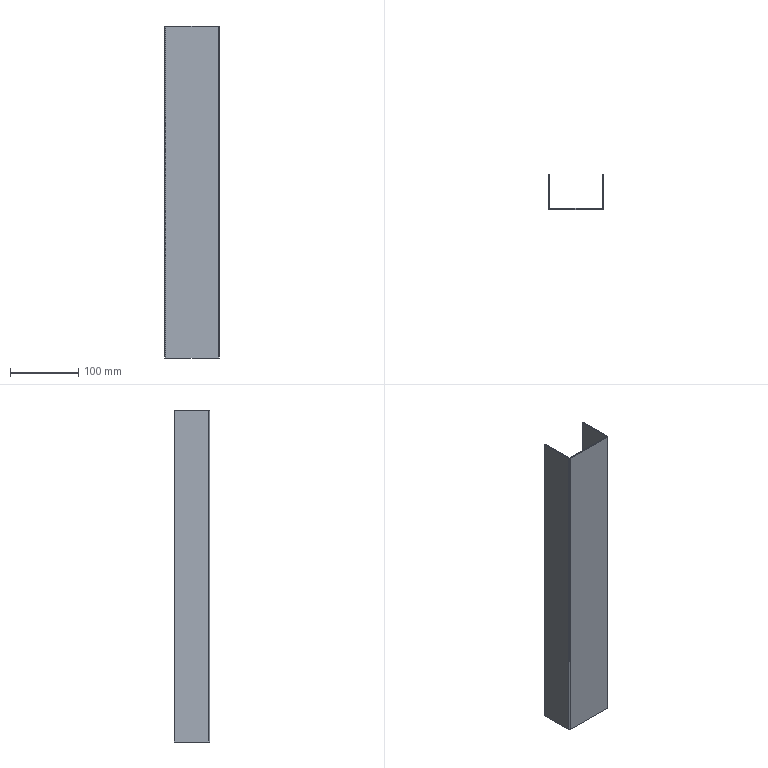Part | SolidWorks | features SplitBody 1 | 1 solid | 22 faces | box 80 x 51.5 x 487 mm | volume 130957 mm3 | plane 18 | cylinder 4 | commonest cylinder face diameters 0.2 x2 3.2 x2
STEP:
#1=CARTESIAN_POINT('',(40.,-51.4,-243.5));
#2=VERTEX_POINT('',#1);
#3=CARTESIAN_POINT('',(38.5,-51.4,-243.5));
#4=VERTEX_POINT('',#3);
#5=CARTESIAN_POINT('',(40.,-51.4,-243.5));
#6=DIRECTION('',(-1.,0.,0.));
#7=VECTOR('',#6,1000.);
#8=LINE('',#5,#7);
#9=EDGE_CURVE('',#2,#4,#8,.T.);
#10=ORIENTED_EDGE('',*,*,#9,.F.);
#11=CARTESIAN_POINT('',(38.4,-53.,-243.5));
#12=VERTEX_POINT('',#11);
#13=CARTESIAN_POINT('',(38.4,-51.4,-243.5));
#14=DIRECTION('',(0.,0.,-1.));
#15=DIRECTION('',(1.,0.,0.));
#16=AXIS2_PLACEMENT_3D('',#13,#14,#15);
#17=CIRCLE('',#16,1.6);
#18=EDGE_CURVE('',#2,#12,#17,.T.);
#19=ORIENTED_EDGE('',*,*,#18,.T.);
#20=CARTESIAN_POINT('',(38.4,-51.5,-243.5));
#21=VERTEX_POINT('',#20);
#22=CARTESIAN_POINT('',(38.4,-51.5,-243.5));
#23=DIRECTION('',(0.,-1.,0.));
#24=VECTOR('',#23,1000.);
#25=LINE('',#22,#24);
#26=EDGE_CURVE('',#21,#12,#25,.T.);
#27=ORIENTED_EDGE('',*,*,#26,.F.);
#28=CARTESIAN_POINT('',(38.4,-51.4,-243.5));
#29=DIRECTION('',(0.,0.,-1.));
#30=DIRECTION('',(1.,0.,0.));
#31=AXIS2_PLACEMENT_3D('',#28,#29,#30);
#32=CIRCLE('',#31,0.1);
#33=EDGE_CURVE('',#4,#21,#32,.T.);
#34=ORIENTED_EDGE('',*,*,#33,.F.);
#35=EDGE_LOOP('',(#10,#19,#27,#34));
#36=FACE_OUTER_BOUND('',#35,.T.);
#37=CARTESIAN_POINT('',(40.,-51.4,-243.5));
#38=DIRECTION('',(0.,0.,-1.));
#39=DIRECTION('',(-1.,0.,0.));
#40=AXIS2_PLACEMENT_3D('',#37,#38,#39);
#41=PLANE('',#40);
#42=ADVANCED_FACE('',(#36),#41,.T.);
#43=CARTESIAN_POINT('',(40.,-1.5,-243.5));
#44=VERTEX_POINT('',#43);
#45=CARTESIAN_POINT('',(40.,-53.,-243.5));
#46=DIRECTION('',(0.,-1.,0.));
#47=VECTOR('',#46,1000.);
#48=LINE('',#45,#47);
#49=EDGE_CURVE('',#44,#2,#48,.T.);
#50=ORIENTED_EDGE('',*,*,#49,.T.);
#51=ORIENTED_EDGE('',*,*,#9,.T.);
#52=CARTESIAN_POINT('',(38.5,-1.5,-243.5));
#53=VERTEX_POINT('',#52);
#54=CARTESIAN_POINT('',(38.5,-53.,-243.5));
#55=DIRECTION('',(0.,-1.,0.));
#56=VECTOR('',#55,1000.);
#57=LINE('',#54,#56);
#58=EDGE_CURVE('',#53,#4,#57,.T.);
#59=ORIENTED_EDGE('',*,*,#58,.F.);
#60=CARTESIAN_POINT('',(38.5,-1.5,-243.5));
#61=DIRECTION('',(1.,0.,0.));
#62=VECTOR('',#61,1000.);
#63=LINE('',#60,#62);
#64=EDGE_CURVE('',#53,#44,#63,.T.);
#65=ORIENTED_EDGE('',*,*,#64,.T.);
#66=EDGE_LOOP('',(#50,#51,#59,#65));
#67=FACE_OUTER_BOUND('',#66,.T.);
#68=CARTESIAN_POINT('',(38.4,-51.5,-243.5));
#69=DIRECTION('',(0.,0.,-1.));
#70=DIRECTION('',(-1.,0.,0.));
#71=AXIS2_PLACEMENT_3D('',#68,#69,#70);
#72=PLANE('',#71);
#73=ADVANCED_FACE('',(#67),#72,.T.);
#74=CARTESIAN_POINT('',(-38.4,-53.,-243.5));
#75=VERTEX_POINT('',#74);
#76=CARTESIAN_POINT('',(-38.4,-51.5,-243.5));
#77=VERTEX_POINT('',#76);
#78=CARTESIAN_POINT('',(-38.4,-53.,-243.5));
#79=DIRECTION('',(0.,1.,0.));
#80=VECTOR('',#79,1000.);
#81=LINE('',#78,#80);
#82=EDGE_CURVE('',#75,#77,#81,.T.);
#83=ORIENTED_EDGE('',*,*,#82,.F.);
#84=CARTESIAN_POINT('',(-40.,-51.4,-243.5));
#85=VERTEX_POINT('',#84);
#86=CARTESIAN_POINT('',(-38.4,-51.4,-243.5));
#87=DIRECTION('',(0.,0.,-1.));
#88=DIRECTION('',(1.,0.,0.));
#89=AXIS2_PLACEMENT_3D('',#86,#87,#88);
#90=CIRCLE('',#89,1.6);
#91=EDGE_CURVE('',#75,#85,#90,.T.);
#92=ORIENTED_EDGE('',*,*,#91,.T.);
#93=CARTESIAN_POINT('',(-38.5,-51.4,-243.5));
#94=VERTEX_POINT('',#93);
#95=CARTESIAN_POINT('',(-38.5,-51.4,-243.5));
#96=DIRECTION('',(-1.,0.,0.));
#97=VECTOR('',#96,1000.);
#98=LINE('',#95,#97);
#99=EDGE_CURVE('',#94,#85,#98,.T.);
#100=ORIENTED_EDGE('',*,*,#99,.F.);
#101=CARTESIAN_POINT('',(-38.4,-51.4,-243.5));
#102=DIRECTION('',(0.,0.,-1.));
#103=DIRECTION('',(1.,0.,0.));
#104=AXIS2_PLACEMENT_3D('',#101,#102,#103);
#105=CIRCLE('',#104,0.1);
#106=EDGE_CURVE('',#77,#94,#105,.T.);
#107=ORIENTED_EDGE('',*,*,#106,.F.);
#108=EDGE_LOOP('',(#83,#92,#100,#107));
#109=FACE_OUTER_BOUND('',#108,.T.);
#110=CARTESIAN_POINT('',(-38.4,-53.,-243.5));
#111=DIRECTION('',(0.,0.,-1.));
#112=DIRECTION('',(-1.,0.,0.));
#113=AXIS2_PLACEMENT_3D('',#110,#111,#112);
#114=PLANE('',#113);
#115=ADVANCED_FACE('',(#109),#114,.T.);
#116=CARTESIAN_POINT('',(-40.,-53.,-243.5));
#117=DIRECTION('',(-1.,0.,0.));
#118=VECTOR('',#117,1000.);
#119=LINE('',#116,#118);
#120=EDGE_CURVE('',#12,#75,#119,.T.);
#121=ORIENTED_EDGE('',*,*,#120,.T.);
#122=ORIENTED_EDGE('',*,*,#82,.T.);
#123=CARTESIAN_POINT('',(-40.,-51.5,-243.5));
#124=DIRECTION('',(-1.,0.,0.));
#125=VECTOR('',#124,1000.);
#126=LINE('',#123,#125);
#127=EDGE_CURVE('',#21,#77,#126,.T.);
#128=ORIENTED_EDGE('',*,*,#127,.F.);
#129=ORIENTED_EDGE('',*,*,#26,.T.);
#130=EDGE_LOOP('',(#121,#122,#128,#129));
#131=FACE_OUTER_BOUND('',#130,.T.);
#132=CARTESIAN_POINT('',(-38.5,-51.4,-243.5));
#133=DIRECTION('',(0.,0.,-1.));
#134=DIRECTION('',(-1.,0.,0.));
#135=AXIS2_PLACEMENT_3D('',#132,#133,#134);
#136=PLANE('',#135);
#137=ADVANCED_FACE('',(#131),#136,.T.);
#138=CARTESIAN_POINT('',(-38.5,-51.4,243.5));
#139=VERTEX_POINT('',#138);
#140=CARTESIAN_POINT('',(-38.5,-1.5,243.5));
#141=VERTEX_POINT('',#140);
#142=CARTESIAN_POINT('',(-38.5,-53.,243.5));
#143=DIRECTION('',(0.,1.,0.));
#144=VECTOR('',#143,1000.);
#145=LINE('',#142,#144);
#146=EDGE_CURVE('',#139,#141,#145,.T.);
#147=ORIENTED_EDGE('',*,*,#146,.F.);
#148=CARTESIAN_POINT('',(-38.5,-51.4,338.643));
#149=DIRECTION('',(0.,0.,-1.));
#150=VECTOR('',#149,1000.);
#151=LINE('',#148,#150);
#152=EDGE_CURVE('',#139,#94,#151,.T.);
#153=ORIENTED_EDGE('',*,*,#152,.T.);
#154=CARTESIAN_POINT('',(-38.5,-1.5,-243.5));
#155=VERTEX_POINT('',#154);
#156=CARTESIAN_POINT('',(-38.5,-53.,-243.5));
#157=DIRECTION('',(0.,1.,0.));
#158=VECTOR('',#157,1000.);
#159=LINE('',#156,#158);
#160=EDGE_CURVE('',#94,#155,#159,.T.);
#161=ORIENTED_EDGE('',*,*,#160,.T.);
#162=CARTESIAN_POINT('',(-38.5,-1.5,338.643));
#163=DIRECTION('',(0.,0.,-1.));
#164=VECTOR('',#163,1000.);
#165=LINE('',#162,#164);
#166=EDGE_CURVE('',#141,#155,#165,.T.);
#167=ORIENTED_EDGE('',*,*,#166,.F.);
#168=EDGE_LOOP('',(#147,#153,#161,#167));
#169=FACE_OUTER_BOUND('',#168,.T.);
#170=CARTESIAN_POINT('',(-38.5,-53.,338.643));
#171=DIRECTION('',(-1.,0.,0.));
#172=DIRECTION('',(0.,-1.,0.));
#173=AXIS2_PLACEMENT_3D('',#170,#171,#172);
#174=PLANE('',#173);
#175=ADVANCED_FACE('',(#169),#174,.F.);
#176=CARTESIAN_POINT('',(-40.,-1.5,243.5));
#177=VERTEX_POINT('',#176);
#178=CARTESIAN_POINT('',(-40.,-1.5,-243.5));
#179=VERTEX_POINT('',#178);
#180=CARTESIAN_POINT('',(-40.,-1.5,338.643));
#181=DIRECTION('',(0.,0.,-1.));
#182=VECTOR('',#181,1000.);
#183=LINE('',#180,#182);
#184=EDGE_CURVE('',#177,#179,#183,.T.);
#185=ORIENTED_EDGE('',*,*,#184,.F.);
#186=CARTESIAN_POINT('',(-40.,-1.5,243.5));
#187=DIRECTION('',(1.,0.,0.));
#188=VECTOR('',#187,1000.);
#189=LINE('',#186,#188);
#190=EDGE_CURVE('',#177,#141,#189,.T.);
#191=ORIENTED_EDGE('',*,*,#190,.T.);
#192=ORIENTED_EDGE('',*,*,#166,.T.);
#193=CARTESIAN_POINT('',(-40.,-1.5,-243.5));
#194=DIRECTION('',(1.,0.,0.));
#195=VECTOR('',#194,1000.);
#196=LINE('',#193,#195);
#197=EDGE_CURVE('',#179,#155,#196,.T.);
#198=ORIENTED_EDGE('',*,*,#197,.F.);
#199=EDGE_LOOP('',(#185,#191,#192,#198));
#200=FACE_OUTER_BOUND('',#199,.T.);
#201=CARTESIAN_POINT('',(-40.,-1.5,338.643));
#202=DIRECTION('',(0.,1.,0.));
#203=DIRECTION('',(-1.,0.,0.));
#204=AXIS2_PLACEMENT_3D('',#201,#202,#203);
#205=PLANE('',#204);
#206=ADVANCED_FACE('',(#200),#205,.T.);
#207=CARTESIAN_POINT('',(-40.,-51.4,243.5));
#208=VERTEX_POINT('',#207);
#209=CARTESIAN_POINT('',(-40.,-51.4,338.643));
#210=DIRECTION('',(0.,0.,-1.));
#211=VECTOR('',#210,1000.);
#212=LINE('',#209,#211);
#213=EDGE_CURVE('',#208,#85,#212,.T.);
#214=ORIENTED_EDGE('',*,*,#213,.F.);
#215=CARTESIAN_POINT('',(-40.,-53.,243.5));
#216=DIRECTION('',(0.,1.,0.));
#217=VECTOR('',#216,1000.);
#218=LINE('',#215,#217);
#219=EDGE_CURVE('',#208,#177,#218,.T.);
#220=ORIENTED_EDGE('',*,*,#219,.T.);
#221=ORIENTED_EDGE('',*,*,#184,.T.);
#222=CARTESIAN_POINT('',(-40.,-53.,-243.5));
#223=DIRECTION('',(0.,1.,0.));
#224=VECTOR('',#223,1000.);
#225=LINE('',#222,#224);
#226=EDGE_CURVE('',#85,#179,#225,.T.);
#227=ORIENTED_EDGE('',*,*,#226,.F.);
#228=EDGE_LOOP('',(#214,#220,#221,#227));
#229=FACE_OUTER_BOUND('',#228,.T.);
#230=CARTESIAN_POINT('',(-40.,-53.,338.643));
#231=DIRECTION('',(-1.,0.,0.));
#232=DIRECTION('',(0.,-1.,0.));
#233=AXIS2_PLACEMENT_3D('',#230,#231,#232);
#234=PLANE('',#233);
#235=ADVANCED_FACE('',(#229),#234,.T.);
#236=CARTESIAN_POINT('',(-38.4,-53.,243.5));
#237=VERTEX_POINT('',#236);
#238=CARTESIAN_POINT('',(-38.4,-53.,338.643));
#239=DIRECTION('',(0.,0.,-1.));
#240=VECTOR('',#239,1000.);
#241=LINE('',#238,#240);
#242=EDGE_CURVE('',#237,#75,#241,.T.);
#243=ORIENTED_EDGE('',*,*,#242,.F.);
#244=CARTESIAN_POINT('',(-38.4,-51.4,243.5));
#245=DIRECTION('',(0.,0.,1.));
#246=DIRECTION('',(0.,1.,0.));
#247=AXIS2_PLACEMENT_3D('',#244,#245,#246);
#248=CIRCLE('',#247,1.6);
#249=EDGE_CURVE('',#208,#237,#248,.T.);
#250=ORIENTED_EDGE('',*,*,#249,.F.);
#251=ORIENTED_EDGE('',*,*,#213,.T.);
#252=ORIENTED_EDGE('',*,*,#91,.F.);
#253=EDGE_LOOP('',(#243,#250,#251,#252));
#254=FACE_OUTER_BOUND('',#253,.T.);
#255=CARTESIAN_POINT('',(-38.4,-51.4,338.643));
#256=DIRECTION('',(0.,0.,-1.));
#257=DIRECTION('',(-1.,0.,0.));
#258=AXIS2_PLACEMENT_3D('',#255,#256,#257);
#259=CYLINDRICAL_SURFACE('',#258,1.6);
#260=ADVANCED_FACE('',(#254),#259,.T.);
#261=CARTESIAN_POINT('',(38.4,-53.,243.5));
#262=VERTEX_POINT('',#261);
#263=CARTESIAN_POINT('',(38.4,-53.,338.643));
#264=DIRECTION('',(0.,0.,-1.));
#265=VECTOR('',#264,1000.);
#266=LINE('',#263,#265);
#267=EDGE_CURVE('',#262,#12,#266,.T.);
#268=ORIENTED_EDGE('',*,*,#267,.F.);
#269=CARTESIAN_POINT('',(-40.,-53.,243.5));
#270=DIRECTION('',(-1.,0.,0.));
#271=VECTOR('',#270,1000.);
#272=LINE('',#269,#271);
#273=EDGE_CURVE('',#262,#237,#272,.T.);
#274=ORIENTED_EDGE('',*,*,#273,.T.);
#275=ORIENTED_EDGE('',*,*,#242,.T.);
#276=ORIENTED_EDGE('',*,*,#120,.F.);
#277=EDGE_LOOP('',(#268,#274,#275,#276));
#278=FACE_OUTER_BOUND('',#277,.T.);
#279=CARTESIAN_POINT('',(-40.,-53.,338.643));
#280=DIRECTION('',(0.,-1.,0.));
#281=DIRECTION('',(1.,0.,0.));
#282=AXIS2_PLACEMENT_3D('',#279,#280,#281);
#283=PLANE('',#282);
#284=ADVANCED_FACE('',(#278),#283,.T.);
#285=CARTESIAN_POINT('',(40.,-51.4,243.5));
#286=VERTEX_POINT('',#285);
#287=CARTESIAN_POINT('',(40.,-51.4,338.643));
#288=DIRECTION('',(0.,0.,-1.));
#289=VECTOR('',#288,1000.);
#290=LINE('',#287,#289);
#291=EDGE_CURVE('',#286,#2,#290,.T.);
#292=ORIENTED_EDGE('',*,*,#291,.F.);
#293=CARTESIAN_POINT('',(38.4,-51.4,243.5));
#294=DIRECTION('',(0.,0.,1.));
#295=DIRECTION('',(0.,1.,0.));
#296=AXIS2_PLACEMENT_3D('',#293,#294,#295);
#297=CIRCLE('',#296,1.6);
#298=EDGE_CURVE('',#262,#286,#297,.T.);
#299=ORIENTED_EDGE('',*,*,#298,.F.);
#300=ORIENTED_EDGE('',*,*,#267,.T.);
#301=ORIENTED_EDGE('',*,*,#18,.F.);
#302=EDGE_LOOP('',(#292,#299,#300,#301));
#303=FACE_OUTER_BOUND('',#302,.T.);
#304=CARTESIAN_POINT('',(38.4,-51.4,338.643));
#305=DIRECTION('',(0.,0.,-1.));
#306=DIRECTION('',(-1.,0.,0.));
#307=AXIS2_PLACEMENT_3D('',#304,#305,#306);
#308=CYLINDRICAL_SURFACE('',#307,1.6);
#309=ADVANCED_FACE('',(#303),#308,.T.);
#310=CARTESIAN_POINT('',(40.,-1.5,243.5));
#311=VERTEX_POINT('',#310);
#312=CARTESIAN_POINT('',(40.,-1.5,338.643));
#313=DIRECTION('',(0.,0.,-1.));
#314=VECTOR('',#313,1000.);
#315=LINE('',#312,#314);
#316=EDGE_CURVE('',#311,#44,#315,.T.);
#317=ORIENTED_EDGE('',*,*,#316,.F.);
#318=CARTESIAN_POINT('',(40.,-53.,243.5));
#319=DIRECTION('',(0.,-1.,0.));
#320=VECTOR('',#319,1000.);
#321=LINE('',#318,#320);
#322=EDGE_CURVE('',#311,#286,#321,.T.);
#323=ORIENTED_EDGE('',*,*,#322,.T.);
#324=ORIENTED_EDGE('',*,*,#291,.T.);
#325=ORIENTED_EDGE('',*,*,#49,.F.);
#326=EDGE_LOOP('',(#317,#323,#324,#325));
#327=FACE_OUTER_BOUND('',#326,.T.);
#328=CARTESIAN_POINT('',(40.,-53.,338.643));
#329=DIRECTION('',(1.,0.,0.));
#330=DIRECTION('',(0.,1.,0.));
#331=AXIS2_PLACEMENT_3D('',#328,#329,#330);
#332=PLANE('',#331);
#333=ADVANCED_FACE('',(#327),#332,.T.);
#334=CARTESIAN_POINT('',(38.5,-1.5,243.5));
#335=VERTEX_POINT('',#334);
#336=CARTESIAN_POINT('',(38.5,-1.5,338.643));
#337=DIRECTION('',(0.,0.,-1.));
#338=VECTOR('',#337,1000.);
#339=LINE('',#336,#338);
#340=EDGE_CURVE('',#335,#53,#339,.T.);
#341=ORIENTED_EDGE('',*,*,#340,.F.);
#342=CARTESIAN_POINT('',(38.5,-1.5,243.5));
#343=DIRECTION('',(1.,0.,0.));
#344=VECTOR('',#343,1000.);
#345=LINE('',#342,#344);
#346=EDGE_CURVE('',#335,#311,#345,.T.);
#347=ORIENTED_EDGE('',*,*,#346,.T.);
#348=ORIENTED_EDGE('',*,*,#316,.T.);
#349=ORIENTED_EDGE('',*,*,#64,.F.);
#350=EDGE_LOOP('',(#341,#347,#348,#349));
#351=FACE_OUTER_BOUND('',#350,.T.);
#352=CARTESIAN_POINT('',(38.5,-1.5,338.643));
#353=DIRECTION('',(0.,1.,0.));
#354=DIRECTION('',(-1.,0.,0.));
#355=AXIS2_PLACEMENT_3D('',#352,#353,#354);
#356=PLANE('',#355);
#357=ADVANCED_FACE('',(#351),#356,.T.);
#358=CARTESIAN_POINT('',(38.5,-51.4,243.5));
#359=VERTEX_POINT('',#358);
#360=CARTESIAN_POINT('',(38.5,-53.,243.5));
#361=DIRECTION('',(0.,-1.,0.));
#362=VECTOR('',#361,1000.);
#363=LINE('',#360,#362);
#364=EDGE_CURVE('',#335,#359,#363,.T.);
#365=ORIENTED_EDGE('',*,*,#364,.F.);
#366=ORIENTED_EDGE('',*,*,#340,.T.);
#367=ORIENTED_EDGE('',*,*,#58,.T.);
#368=CARTESIAN_POINT('',(38.5,-51.4,338.643));
#369=DIRECTION('',(0.,0.,-1.));
#370=VECTOR('',#369,1000.);
#371=LINE('',#368,#370);
#372=EDGE_CURVE('',#359,#4,#371,.T.);
#373=ORIENTED_EDGE('',*,*,#372,.F.);
#374=EDGE_LOOP('',(#365,#366,#367,#373));
#375=FACE_OUTER_BOUND('',#374,.T.);
#376=CARTESIAN_POINT('',(38.5,-53.,338.643));
#377=DIRECTION('',(1.,0.,0.));
#378=DIRECTION('',(0.,1.,0.));
#379=AXIS2_PLACEMENT_3D('',#376,#377,#378);
#380=PLANE('',#379);
#381=ADVANCED_FACE('',(#375),#380,.F.);
#382=CARTESIAN_POINT('',(38.4,-51.5,243.5));
#383=VERTEX_POINT('',#382);
#384=CARTESIAN_POINT('',(38.4,-51.4,243.5));
#385=DIRECTION('',(0.,0.,-1.));
#386=DIRECTION('',(0.,-1.,0.));
#387=AXIS2_PLACEMENT_3D('',#384,#385,#386);
#388=CIRCLE('',#387,0.1);
#389=EDGE_CURVE('',#359,#383,#388,.T.);
#390=ORIENTED_EDGE('',*,*,#389,.F.);
#391=ORIENTED_EDGE('',*,*,#372,.T.);
#392=ORIENTED_EDGE('',*,*,#33,.T.);
#393=CARTESIAN_POINT('',(38.4,-51.5,338.643));
#394=DIRECTION('',(0.,0.,-1.));
#395=VECTOR('',#394,1000.);
#396=LINE('',#393,#395);
#397=EDGE_CURVE('',#383,#21,#396,.T.);
#398=ORIENTED_EDGE('',*,*,#397,.F.);
#399=EDGE_LOOP('',(#390,#391,#392,#398));
#400=FACE_OUTER_BOUND('',#399,.T.);
#401=CARTESIAN_POINT('',(38.4,-51.4,338.643));
#402=DIRECTION('',(0.,0.,-1.));
#403=DIRECTION('',(-1.,0.,0.));
#404=AXIS2_PLACEMENT_3D('',#401,#402,#403);
#405=CYLINDRICAL_SURFACE('',#404,0.1);
#406=ADVANCED_FACE('',(#400),#405,.F.);
#407=CARTESIAN_POINT('',(-38.4,-51.5,243.5));
#408=VERTEX_POINT('',#407);
#409=CARTESIAN_POINT('',(-40.,-51.5,243.5));
#410=DIRECTION('',(-1.,0.,0.));
#411=VECTOR('',#410,1000.);
#412=LINE('',#409,#411);
#413=EDGE_CURVE('',#383,#408,#412,.T.);
#414=ORIENTED_EDGE('',*,*,#413,.F.);
#415=ORIENTED_EDGE('',*,*,#397,.T.);
#416=ORIENTED_EDGE('',*,*,#127,.T.);
#417=CARTESIAN_POINT('',(-38.4,-51.5,338.643));
#418=DIRECTION('',(0.,0.,-1.));
#419=VECTOR('',#418,1000.);
#420=LINE('',#417,#419);
#421=EDGE_CURVE('',#408,#77,#420,.T.);
#422=ORIENTED_EDGE('',*,*,#421,.F.);
#423=EDGE_LOOP('',(#414,#415,#416,#422));
#424=FACE_OUTER_BOUND('',#423,.T.);
#425=CARTESIAN_POINT('',(-40.,-51.5,338.643));
#426=DIRECTION('',(0.,-1.,0.));
#427=DIRECTION('',(1.,0.,0.));
#428=AXIS2_PLACEMENT_3D('',#425,#426,#427);
#429=PLANE('',#428);
#430=ADVANCED_FACE('',(#424),#429,.F.);
#431=CARTESIAN_POINT('',(-38.4,-51.4,243.5));
#432=DIRECTION('',(0.,0.,-1.));
#433=DIRECTION('',(0.,-1.,0.));
#434=AXIS2_PLACEMENT_3D('',#431,#432,#433);
#435=CIRCLE('',#434,0.1);
#436=EDGE_CURVE('',#408,#139,#435,.T.);
#437=ORIENTED_EDGE('',*,*,#436,.F.);
#438=ORIENTED_EDGE('',*,*,#421,.T.);
#439=ORIENTED_EDGE('',*,*,#106,.T.);
#440=ORIENTED_EDGE('',*,*,#152,.F.);
#441=EDGE_LOOP('',(#437,#438,#439,#440));
#442=FACE_OUTER_BOUND('',#441,.T.);
#443=CARTESIAN_POINT('',(-38.4,-51.4,338.643));
#444=DIRECTION('',(0.,0.,-1.));
#445=DIRECTION('',(-1.,0.,0.));
#446=AXIS2_PLACEMENT_3D('',#443,#444,#445);
#447=CYLINDRICAL_SURFACE('',#446,0.1);
#448=ADVANCED_FACE('',(#442),#447,.F.);
#449=ORIENTED_EDGE('',*,*,#160,.F.);
#450=ORIENTED_EDGE('',*,*,#99,.T.);
#451=ORIENTED_EDGE('',*,*,#226,.T.);
#452=ORIENTED_EDGE('',*,*,#197,.T.);
#453=EDGE_LOOP('',(#449,#450,#451,#452));
#454=FACE_OUTER_BOUND('',#453,.T.);
#455=CARTESIAN_POINT('',(-38.4,-51.4,-243.5));
#456=DIRECTION('',(0.,0.,1.));
#457=DIRECTION('',(1.,0.,0.));
#458=AXIS2_PLACEMENT_3D('',#455,#456,#457);
#459=PLANE('',#458);
#460=ADVANCED_FACE('',(#454),#459,.F.);
#461=ORIENTED_EDGE('',*,*,#413,.T.);
#462=CARTESIAN_POINT('',(-38.4,-51.5,243.5));
#463=DIRECTION('',(0.,-1.,0.));
#464=VECTOR('',#463,1000.);
#465=LINE('',#462,#464);
#466=EDGE_CURVE('',#408,#237,#465,.T.);
#467=ORIENTED_EDGE('',*,*,#466,.T.);
#468=ORIENTED_EDGE('',*,*,#273,.F.);
#469=CARTESIAN_POINT('',(38.4,-51.5,243.5));
#470=DIRECTION('',(0.,-1.,0.));
#471=VECTOR('',#470,1000.);
#472=LINE('',#469,#471);
#473=EDGE_CURVE('',#383,#262,#472,.T.);
#474=ORIENTED_EDGE('',*,*,#473,.F.);
#475=EDGE_LOOP('',(#461,#467,#468,#474));
#476=FACE_OUTER_BOUND('',#475,.T.);
#477=CARTESIAN_POINT('',(-40.,-51.5,243.5));
#478=DIRECTION('',(0.,0.,1.));
#479=DIRECTION('',(-1.,0.,0.));
#480=AXIS2_PLACEMENT_3D('',#477,#478,#479);
#481=PLANE('',#480);
#482=ADVANCED_FACE('',(#476),#481,.T.);
#483=ORIENTED_EDGE('',*,*,#364,.T.);
#484=CARTESIAN_POINT('',(38.5,-51.4,243.5));
#485=DIRECTION('',(1.,0.,0.));
#486=VECTOR('',#485,1000.);
#487=LINE('',#484,#486);
#488=EDGE_CURVE('',#359,#286,#487,.T.);
#489=ORIENTED_EDGE('',*,*,#488,.T.);
#490=ORIENTED_EDGE('',*,*,#322,.F.);
#491=ORIENTED_EDGE('',*,*,#346,.F.);
#492=EDGE_LOOP('',(#483,#489,#490,#491));
#493=FACE_OUTER_BOUND('',#492,.T.);
#494=CARTESIAN_POINT('',(38.5,-53.,243.5));
#495=DIRECTION('',(0.,0.,1.));
#496=DIRECTION('',(0.,-1.,0.));
#497=AXIS2_PLACEMENT_3D('',#494,#495,#496);
#498=PLANE('',#497);
#499=ADVANCED_FACE('',(#493),#498,.T.);
#500=ORIENTED_EDGE('',*,*,#298,.T.);
#501=ORIENTED_EDGE('',*,*,#488,.F.);
#502=ORIENTED_EDGE('',*,*,#389,.T.);
#503=ORIENTED_EDGE('',*,*,#473,.T.);
#504=EDGE_LOOP('',(#500,#501,#502,#503));
#505=FACE_OUTER_BOUND('',#504,.T.);
#506=CARTESIAN_POINT('',(38.4,-51.4,243.5));
#507=DIRECTION('',(0.,0.,-1.));
#508=DIRECTION('',(0.,1.,0.));
#509=AXIS2_PLACEMENT_3D('',#506,#507,#508);
#510=PLANE('',#509);
#511=ADVANCED_FACE('',(#505),#510,.F.);
#512=ORIENTED_EDGE('',*,*,#190,.F.);
#513=ORIENTED_EDGE('',*,*,#219,.F.);
#514=CARTESIAN_POINT('',(-40.,-51.4,243.5));
#515=DIRECTION('',(1.,0.,0.));
#516=VECTOR('',#515,1000.);
#517=LINE('',#514,#516);
#518=EDGE_CURVE('',#208,#139,#517,.T.);
#519=ORIENTED_EDGE('',*,*,#518,.T.);
#520=ORIENTED_EDGE('',*,*,#146,.T.);
#521=EDGE_LOOP('',(#512,#513,#519,#520));
#522=FACE_OUTER_BOUND('',#521,.T.);
#523=CARTESIAN_POINT('',(-40.,-53.,243.5));
#524=DIRECTION('',(0.,0.,1.));
#525=DIRECTION('',(0.,1.,0.));
#526=AXIS2_PLACEMENT_3D('',#523,#524,#525);
#527=PLANE('',#526);
#528=ADVANCED_FACE('',(#522),#527,.T.);
#529=ORIENTED_EDGE('',*,*,#249,.T.);
#530=ORIENTED_EDGE('',*,*,#466,.F.);
#531=ORIENTED_EDGE('',*,*,#436,.T.);
#532=ORIENTED_EDGE('',*,*,#518,.F.);
#533=EDGE_LOOP('',(#529,#530,#531,#532));
#534=FACE_OUTER_BOUND('',#533,.T.);
#535=CARTESIAN_POINT('',(-38.4,-51.4,243.5));
#536=DIRECTION('',(0.,0.,-1.));
#537=DIRECTION('',(0.,1.,0.));
#538=AXIS2_PLACEMENT_3D('',#535,#536,#537);
#539=PLANE('',#538);
#540=ADVANCED_FACE('',(#534),#539,.F.);
#541=CLOSED_SHELL('',(#42,#73,#115,#137,#175,#206,#235,#260,#284,#309,#333,#357,#381,#406,#430,#448,#460,#482,#499,#511,#528,#540));
#542=MANIFOLD_SOLID_BREP('',#541);
#543=CARTESIAN_POINT('',(0.,0.,0.));
#544=DIRECTION('',(0.,0.,1.));
#545=DIRECTION('',(1.,0.,0.));
#546=AXIS2_PLACEMENT_3D('',#543,#544,#545);
#547=(LENGTH_UNIT()NAMED_UNIT(*)SI_UNIT(.MILLI.,.METRE.));
#548=UNCERTAINTY_MEASURE_WITH_UNIT(LENGTH_MEASURE(0.00001),#547,'','');
#549=(NAMED_UNIT(*)PLANE_ANGLE_UNIT()SI_UNIT($,.RADIAN.));
#550=(NAMED_UNIT(*)SI_UNIT($,.STERADIAN.)SOLID_ANGLE_UNIT());
#551=(GEOMETRIC_REPRESENTATION_CONTEXT(3)GLOBAL_UNCERTAINTY_ASSIGNED_CONTEXT((#548))GLOBAL_UNIT_ASSIGNED_CONTEXT((#547,#549,#550))REPRESENTATION_CONTEXT('',''));
#552=ADVANCED_BREP_SHAPE_REPRESENTATION('',(#542,#546),#551);